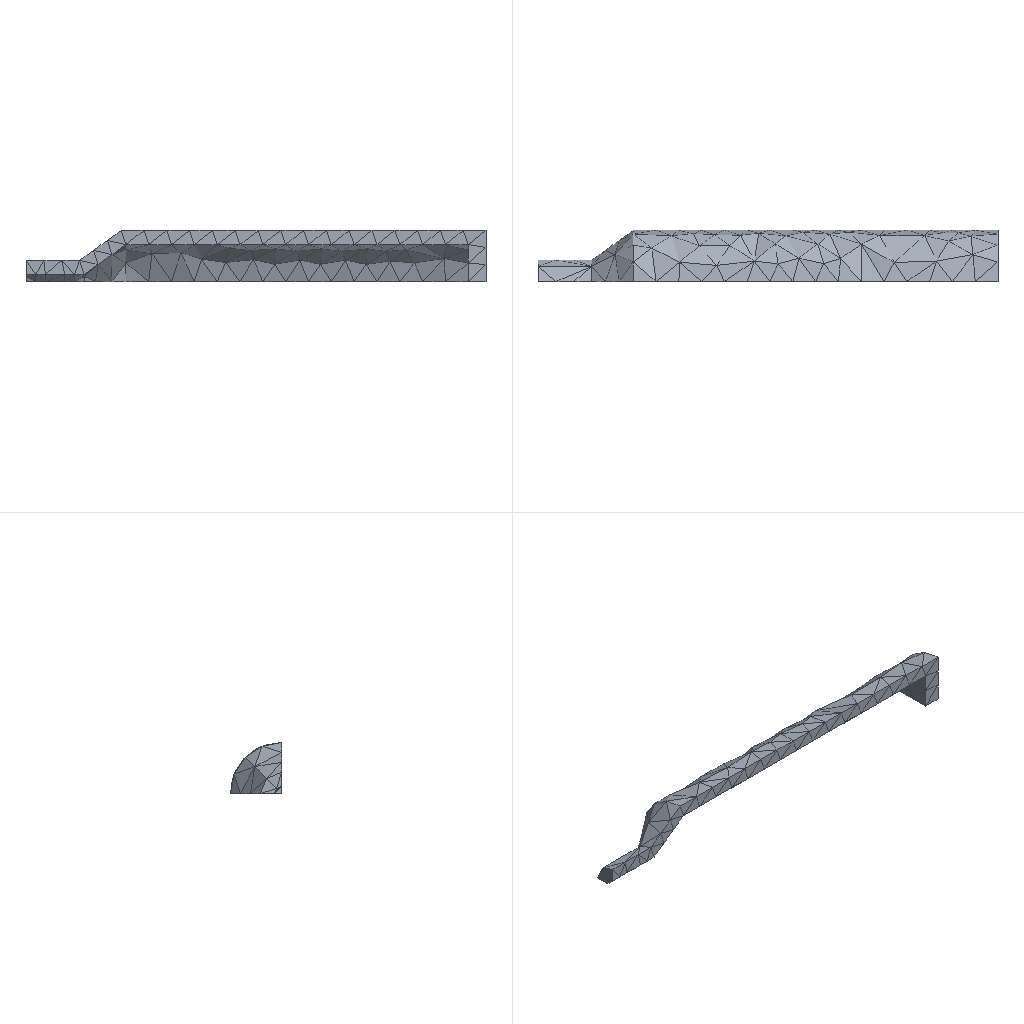Simulation study | ansys workbench
Ansys APDL input file, long lists of numbers shortened:
/batch
/config,noeldb,1     ! force off writing results to database
*get,_wallstrt,active,,time,wall
! ANSYS input file written by Workbench version 2022 R1
! File used for geometry attach:
/title,3--____ (C5)
! ****** Begin Custom Load Command Snippet ******
/COM, ACT Extensions:
/COM,     LSDYNA, 2021.1
/COM,
! ****** End   Custom Load Command Snippet ******
*DIM,_wb_ProjectScratch_dir,string,248
_wb_ProjectScratch_dir(1) = ''
*DIM,_wb_SolverFiles_dir,string,248
_wb_SolverFiles_dir(1) = ''
*DIM,_wb_userfiles_dir,string,248
_wb_userfiles_dir(1) = ''
/com,--- Data in consistent NMM units. See Solving Units in the help system for more information.
/units,MPA
/nopr
/wb,file,start              !  signify a WB generated input file
/prep7
! Turn off shape checking because checks already performed inside WB mesher.
! See help system for more information.
SHPP,OFF,,NOWARN
/nolist
etcon,set             ! allow ANSYS to choose best KEYOP's for 180x elements, resets any applicable keyopt to MAPDL defaults
/com,*********** Nodes for the whole assembly ***********
nblock,3,,946
(1i9,3e20.9e3)
        1     1.299000000E+03     0.000000000E+00     1.443258926E+02
! (859 more lines like these left out)
-1
/wb,elem,start            !  set before creation of elements
/com,*********** Elements for Body 1 "__3-FreeParts|__-__1" ***********
et,1,187
eblock,19,solid,,353
(19i9)
        1        1        1        1        0        0        0        0       10        0        1       41      106      143       42      385      663      387      383
! (705 more lines like these left out)
-1
/wb,elem,end               !  done creating elements
/com,*********** Send User Defined Coordinate System(s) ***********
csys,0
toffst,273.15,  ! Temperature offset from absolute zero
/com,*********** Set Reference Temperature ***********
tref,22.
/wb,mat,start              !  starting to send materials
/com,*********** Send Materials ***********
Temperature = 'TEMP' ! Temperature
MP,DENS,1,7.85e-09,	! tonne mm^-3
MP,ALPX,1,1.2e-05,	! C^-1
MP,C,1,434000000,	! mm^2 s^-2 C^-1
MP,KXX,1,60.5,	! tonne mm s^-3 C^-1
MP,RSVX,1,0.00017,	! ohm mm
MP,EX,1,200000,	! tonne s^-2 mm^-1
MP,NUXY,1,0.3,
MP,MURX,1,10000,
/wb,mat,end                !  done sending materials
!************************* Model Summary ********************
!__3-FreeParts|__-__1,	结构钢,	matid,	1
!************************* End Model Summary ********************
! get the diagonal of the bounding box. Needed later for other things
*get,_xmin,node,,mnloc,x
*get,_ymin,node,,mnloc,y
*get,_zmin,node,,mnloc,z
*get,_xmax,node,,mxloc,x
*get,_ymax,node,,mxloc,y
*get,_zmax,node,,mxloc,z
_ASMDIAG=(_xmax-_xmin)*(_xmax-_xmin)+(_ymax-_ymin)*(_ymax-_ymin)+(_zmax-_zmin)*(_zmax-_zmin)
_ASMDIAG=SQRT(_ASMDIAG)
/wb,contact,start          !  starting to send contact
/wb,contact,end            !  done creating contacts
/golist
/wb,load,start             !  starting to send loads
/com,*********** Fixed Supports ***********
CMBLOCK,_FIXEDSU,NODE,       27
(8i10)
         1         2         3         4         5         6         7         8
         9        10       171       172       175       176       178       179
       180       184       185       191       192       195       196       200
       201       205       210
cmsel,s,_FIXEDSU
d,all,all
nsel,all
/com,*********** Define Pressure Using Surface Effect Elements "__" ***********
et,2,154
eblock,10,,,100
(15i9)
      690        2        2        2        0        8        9      140      140      205      213      140      209
! (99 more lines like these left out)
-1
esel,s,type,,2
keyop,2,7,0                ! Use deformed area for application of load
esel,all
/com,*********** Define Pressure Using Surface Effect Elements "__ 2" ***********
et,3,154
eblock,10,,,78
(15i9)
      790        3        3        3        0       73       74       96       96      525      530       96      527
! (77 more lines like these left out)
-1
esel,s,type,,3
keyop,3,7,0                ! Use deformed area for application of load
esel,all
esel,all
/gst,on,on
fini
*get,_numnode,node,0,count
*get,_numelem,elem,0,count
*get, _MAXELEMNUM, elem, 0, NUM, MAX
*get, _MAXNODENUM, node, 0, NUM, MAX
*get, _MAXELEMTYPE, etyp, 0, NUM, MAX
*get, _MAXREALCONST, real, 0, NUM, MAX
/go
/wb,load,end               !  done creating loads
/com,--- Number of total nodes = %_numnode%
/com,--- Number of contact elements = 178
/com,--- Number of spring elements = 0
/com,--- Number of bearing elements = 0
/com,--- Number of solid elements = 353
/com,--- Number of condensed parts = 0
/com,--- Number of total elements = %_numelem%
*get,_wallbsol,active,,time,wall
/com,****************************************************************************
/com,*************************    SOLUTION       ********************************
/com,****************************************************************************
/solu
antype,0                   ! static analysis
_thickRatio=  0     ! Ratio of thick parts in the model
eqsl,sparse,,,,,1
cntr,print,1               ! print out contact info and also make no initial contact an error
dmpoption,emat,no             ! Don't combine emat file for DANSYS
dmpoption,esav,no             ! Don't combine esav file for DANSYS
nldiag,cont,iter           ! print out contact info each equilibrium iteration
rescontrol,,none                 ! Do not keep any restart files
/com,****************************************************
/com,******************* SOLVE FOR LS 1 OF 1 ****************
esel,s,type,,2
nsle
sf,all,pres,20.
esel,s,type,,3
nsle
sf,all,pres,60.
nsel,all
esel,all
esel,all
/nopr
/gopr
nsub,1,1,1
time,1.
outres,erase
outres,all,none
outres,nsol,all,
outres,rsol,all
outres,eangl,all
outres,etmp,all
outres,veng,all
outres,strs,all,
outres,epel,all,
outres,eppl,all,
outres,cont,all,
! *********** WB SOLVE COMMAND ***********
! check interactive state
*get,ANSINTER_,active,,int
*if,ANSINTER_,ne,0,then
/eof
*endif
solve
/com *************** Write FE CONNECTORS *********
CEWRITE,file,ce,,INTE
/com,****************************************************
/com,*************** FINISHED SOLVE FOR LS 1 *************
*get,_wallasol,active,,time,wall
/nopr
*get,_numnode,node,0,count
*get,_numelem,elem,0,count
*get, _MAXELEMNUM, elem, 0, NUM, MAX
*get, _MAXNODENUM, node, 0, NUM, MAX,,,INTERNAL
*get, _MAXELEMTYPE, etyp, 0, NUM, MAX
*get, _MAXREALCONST, real, 0, NUM, MAX
/gopr
/post1
xmlo,ENCODING,ISO-8859-1
xmlo,parm
/xml,parm,xml
fini
/gopr
*get,_walldone,active,,time,wall
_preptime=(_wallbsol-_wallstrt)*3600
_solvtime=(_wallasol-_wallbsol)*3600
_posttime=(_walldone-_wallasol)*3600
_totaltim=(_walldone-_wallstrt)*3600
*get,_dlbratio,active,0,solu,dlbr
*get,_combtime,active,0,solu,comb
*get,_ssmode,active,0,solu,ssmm
*get,_ndofs,active,0,solu,ndof
*get,_sol_end_time,active,0,set,time
*if,_sol_end_time,eq,1.,then
/fclean				!clean distributed files
*endif
/com,--- Total number of nodes = %_numnode%
/com,--- Total number of elements = %_numelem%
/com,--- Element load balance ratio = %_dlbratio%
/com,--- Time to combine distributed files = %_combtime%
/com,--- Sparse memory mode = %_ssmode%
/com,--- Number of DOF = %_ndofs%
/wb,file,end               ! done with WB generated input